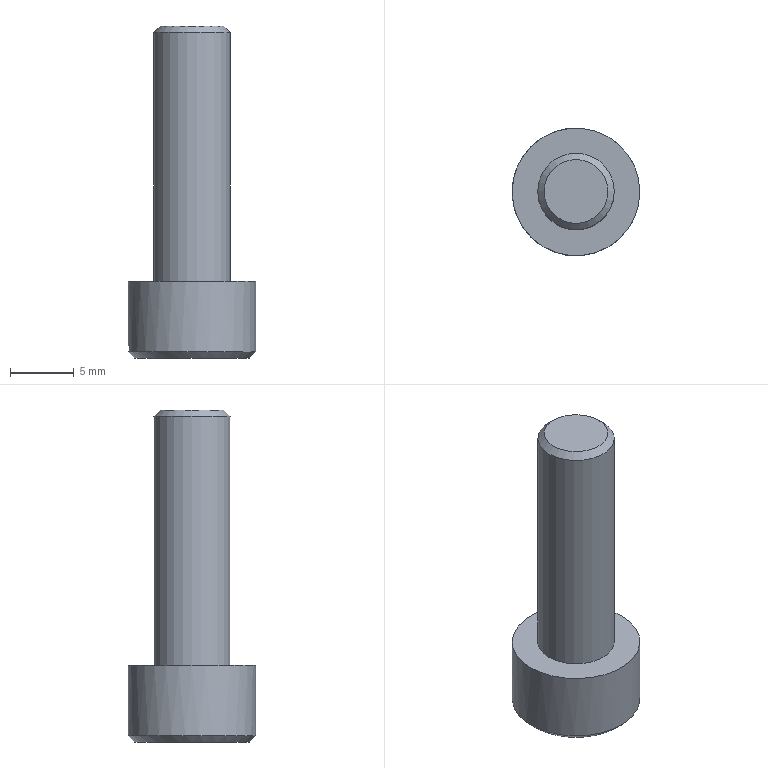Part | STEP file | gslz 2016.10.28-6_id258_x_t | 1 solid | 14 faces | box 10 x 10 x 26 mm | volume 944.102 mm3 | plane 10 | cylinder 2 | cone 2 | commonest cylinder face diameters 6 x1 10 x1
STEP:
#1=CARTESIAN_POINT('',(-78.45,150.,90.992));
#2=VERTEX_POINT('',#1);
#3=CARTESIAN_POINT('',(-82.95,150.,90.992));
#4=DIRECTION('',(0.,0.,1.));
#5=DIRECTION('',(1.,0.,0.));
#6=AXIS2_PLACEMENT_3D('',#3,#4,#5);
#7=CIRCLE('',#6,4.5);
#8=EDGE_CURVE('',#2,#2,#7,.T.);
#9=ORIENTED_EDGE('',*,*,#8,.F.);
#10=EDGE_LOOP('',(#9));
#11=FACE_BOUND('',#10,.T.);
#12=CARTESIAN_POINT('',(-85.45,151.443,90.992));
#13=VERTEX_POINT('',#12);
#14=CARTESIAN_POINT('',(-85.45,148.557,90.992));
#15=VERTEX_POINT('',#14);
#16=CARTESIAN_POINT('',(-85.45,151.443,90.992));
#17=DIRECTION('',(0.,-1.,0.));
#18=VECTOR('',#17,1.);
#19=LINE('',#16,#18);
#20=EDGE_CURVE('',#13,#15,#19,.T.);
#21=ORIENTED_EDGE('',*,*,#20,.T.);
#22=CARTESIAN_POINT('',(-82.95,147.113,90.992));
#23=VERTEX_POINT('',#22);
#24=CARTESIAN_POINT('',(-85.45,148.557,90.992));
#25=DIRECTION('',(0.866,-0.5,0.));
#26=VECTOR('',#25,1.);
#27=LINE('',#24,#26);
#28=EDGE_CURVE('',#15,#23,#27,.T.);
#29=ORIENTED_EDGE('',*,*,#28,.T.);
#30=CARTESIAN_POINT('',(-80.45,148.557,90.992));
#31=VERTEX_POINT('',#30);
#32=CARTESIAN_POINT('',(-82.95,147.113,90.992));
#33=DIRECTION('',(0.866,0.5,0.));
#34=VECTOR('',#33,1.);
#35=LINE('',#32,#34);
#36=EDGE_CURVE('',#23,#31,#35,.T.);
#37=ORIENTED_EDGE('',*,*,#36,.T.);
#38=CARTESIAN_POINT('',(-80.45,151.443,90.992));
#39=VERTEX_POINT('',#38);
#40=CARTESIAN_POINT('',(-80.45,148.557,90.992));
#41=DIRECTION('',(0.,1.,0.));
#42=VECTOR('',#41,1.);
#43=LINE('',#40,#42);
#44=EDGE_CURVE('',#31,#39,#43,.T.);
#45=ORIENTED_EDGE('',*,*,#44,.T.);
#46=CARTESIAN_POINT('',(-82.95,152.887,90.992));
#47=VERTEX_POINT('',#46);
#48=CARTESIAN_POINT('',(-80.45,151.443,90.992));
#49=DIRECTION('',(-0.866,0.5,0.));
#50=VECTOR('',#49,1.);
#51=LINE('',#48,#50);
#52=EDGE_CURVE('',#39,#47,#51,.T.);
#53=ORIENTED_EDGE('',*,*,#52,.T.);
#54=CARTESIAN_POINT('',(-82.95,152.887,90.992));
#55=DIRECTION('',(-0.866,-0.5,0.));
#56=VECTOR('',#55,1.);
#57=LINE('',#54,#56);
#58=EDGE_CURVE('',#47,#13,#57,.T.);
#59=ORIENTED_EDGE('',*,*,#58,.T.);
#60=EDGE_LOOP('',(#21,#29,#37,#45,#53,#59));
#61=FACE_BOUND('',#60,.T.);
#62=CARTESIAN_POINT('',(-82.95,150.,90.992));
#63=DIRECTION('',(0.,0.,-1.));
#64=DIRECTION('',(-1.,0.,0.));
#65=AXIS2_PLACEMENT_3D('',#62,#63,#64);
#66=PLANE('',#65);
#67=ADVANCED_FACE('',(#11,#61),#66,.T.);
#68=CARTESIAN_POINT('',(-85.45,150.,116.992));
#69=VERTEX_POINT('',#68);
#70=CARTESIAN_POINT('',(-82.95,150.,116.992));
#71=DIRECTION('',(0.,0.,-1.));
#72=DIRECTION('',(-1.,0.,0.));
#73=AXIS2_PLACEMENT_3D('',#70,#71,#72);
#74=CIRCLE('',#73,2.5);
#75=EDGE_CURVE('',#69,#69,#74,.T.);
#76=ORIENTED_EDGE('',*,*,#75,.F.);
#77=EDGE_LOOP('',(#76));
#78=FACE_OUTER_BOUND('',#77,.T.);
#79=CARTESIAN_POINT('',(-82.95,150.,116.992));
#80=DIRECTION('',(0.,0.,1.));
#81=DIRECTION('',(1.,0.,0.));
#82=AXIS2_PLACEMENT_3D('',#79,#80,#81);
#83=PLANE('',#82);
#84=ADVANCED_FACE('',(#78),#83,.T.);
#85=CARTESIAN_POINT('',(-79.95,150.,116.492));
#86=VERTEX_POINT('',#85);
#87=CARTESIAN_POINT('',(-82.95,150.,116.492));
#88=DIRECTION('',(0.,0.,1.));
#89=DIRECTION('',(1.,0.,0.));
#90=AXIS2_PLACEMENT_3D('',#87,#88,#89);
#91=CIRCLE('',#90,3.);
#92=EDGE_CURVE('',#86,#86,#91,.T.);
#93=ORIENTED_EDGE('',*,*,#92,.F.);
#94=EDGE_LOOP('',(#93));
#95=FACE_BOUND('',#94,.T.);
#96=CARTESIAN_POINT('',(-85.95,150.,96.992));
#97=VERTEX_POINT('',#96);
#98=CARTESIAN_POINT('',(-82.95,150.,96.992));
#99=DIRECTION('',(0.,0.,-1.));
#100=DIRECTION('',(-1.,0.,0.));
#101=AXIS2_PLACEMENT_3D('',#98,#99,#100);
#102=CIRCLE('',#101,3.);
#103=EDGE_CURVE('',#97,#97,#102,.T.);
#104=ORIENTED_EDGE('',*,*,#103,.F.);
#105=EDGE_LOOP('',(#104));
#106=FACE_BOUND('',#105,.T.);
#107=CARTESIAN_POINT('',(-82.95,150.,108.992));
#108=DIRECTION('',(0.,0.,1.));
#109=DIRECTION('',(1.,0.,0.));
#110=AXIS2_PLACEMENT_3D('',#107,#108,#109);
#111=CYLINDRICAL_SURFACE('',#110,3.);
#112=ADVANCED_FACE('',(#95,#106),#111,.T.);
#113=ORIENTED_EDGE('',*,*,#103,.T.);
#114=EDGE_LOOP('',(#113));
#115=FACE_BOUND('',#114,.T.);
#116=CARTESIAN_POINT('',(-87.95,150.,96.992));
#117=VERTEX_POINT('',#116);
#118=CARTESIAN_POINT('',(-82.95,150.,96.992));
#119=DIRECTION('',(0.,0.,-1.));
#120=DIRECTION('',(-1.,0.,0.));
#121=AXIS2_PLACEMENT_3D('',#118,#119,#120);
#122=CIRCLE('',#121,5.);
#123=EDGE_CURVE('',#117,#117,#122,.T.);
#124=ORIENTED_EDGE('',*,*,#123,.F.);
#125=EDGE_LOOP('',(#124));
#126=FACE_BOUND('',#125,.T.);
#127=CARTESIAN_POINT('',(-82.95,150.,96.992));
#128=DIRECTION('',(0.,0.,1.));
#129=DIRECTION('',(1.,0.,0.));
#130=AXIS2_PLACEMENT_3D('',#127,#128,#129);
#131=PLANE('',#130);
#132=ADVANCED_FACE('',(#115,#126),#131,.T.);
#133=CARTESIAN_POINT('',(-77.95,150.,91.492));
#134=VERTEX_POINT('',#133);
#135=CARTESIAN_POINT('',(-82.95,150.,91.492));
#136=DIRECTION('',(0.,0.,-1.));
#137=DIRECTION('',(1.,0.,0.));
#138=AXIS2_PLACEMENT_3D('',#135,#136,#137);
#139=CIRCLE('',#138,5.);
#140=EDGE_CURVE('',#134,#134,#139,.T.);
#141=ORIENTED_EDGE('',*,*,#140,.F.);
#142=EDGE_LOOP('',(#141));
#143=FACE_BOUND('',#142,.T.);
#144=ORIENTED_EDGE('',*,*,#123,.T.);
#145=EDGE_LOOP('',(#144));
#146=FACE_BOUND('',#145,.T.);
#147=CARTESIAN_POINT('',(-82.95,150.,88.992));
#148=DIRECTION('',(0.,0.,1.));
#149=DIRECTION('',(1.,0.,0.));
#150=AXIS2_PLACEMENT_3D('',#147,#148,#149);
#151=CYLINDRICAL_SURFACE('',#150,5.);
#152=ADVANCED_FACE('',(#143,#146),#151,.T.);
#153=ORIENTED_EDGE('',*,*,#92,.T.);
#154=EDGE_LOOP('',(#153));
#155=FACE_BOUND('',#154,.T.);
#156=ORIENTED_EDGE('',*,*,#75,.T.);
#157=EDGE_LOOP('',(#156));
#158=FACE_BOUND('',#157,.T.);
#159=CARTESIAN_POINT('',(-82.95,150.,116.992));
#160=DIRECTION('',(0.,0.,-1.));
#161=DIRECTION('',(1.,0.,0.));
#162=AXIS2_PLACEMENT_3D('',#159,#160,#161);
#163=CONICAL_SURFACE('',#162,2.5,45.);
#164=ADVANCED_FACE('',(#155,#158),#163,.T.);
#165=ORIENTED_EDGE('',*,*,#20,.F.);
#166=CARTESIAN_POINT('',(-85.45,151.443,94.992));
#167=VERTEX_POINT('',#166);
#168=CARTESIAN_POINT('',(-85.45,151.443,94.992));
#169=DIRECTION('',(0.,0.,1.));
#170=VECTOR('',#169,1.);
#171=LINE('',#168,#170);
#172=EDGE_CURVE('',#13,#167,#171,.T.);
#173=ORIENTED_EDGE('',*,*,#172,.T.);
#174=CARTESIAN_POINT('',(-85.45,148.557,94.992));
#175=VERTEX_POINT('',#174);
#176=CARTESIAN_POINT('',(-85.45,151.443,94.992));
#177=DIRECTION('',(0.,1.,0.));
#178=VECTOR('',#177,1.);
#179=LINE('',#176,#178);
#180=EDGE_CURVE('',#175,#167,#179,.T.);
#181=ORIENTED_EDGE('',*,*,#180,.F.);
#182=CARTESIAN_POINT('',(-85.45,148.557,94.992));
#183=DIRECTION('',(0.,0.,1.));
#184=VECTOR('',#183,1.);
#185=LINE('',#182,#184);
#186=EDGE_CURVE('',#15,#175,#185,.T.);
#187=ORIENTED_EDGE('',*,*,#186,.F.);
#188=EDGE_LOOP('',(#165,#173,#181,#187));
#189=FACE_OUTER_BOUND('',#188,.T.);
#190=CARTESIAN_POINT('',(-85.45,151.443,94.992));
#191=DIRECTION('',(-1.,0.,0.));
#192=DIRECTION('',(0.,0.,1.));
#193=AXIS2_PLACEMENT_3D('',#190,#191,#192);
#194=PLANE('',#193);
#195=ADVANCED_FACE('',(#189),#194,.F.);
#196=ORIENTED_EDGE('',*,*,#28,.F.);
#197=ORIENTED_EDGE('',*,*,#186,.T.);
#198=CARTESIAN_POINT('',(-82.95,147.113,94.992));
#199=VERTEX_POINT('',#198);
#200=CARTESIAN_POINT('',(-85.45,148.557,94.992));
#201=DIRECTION('',(-0.866,0.5,0.));
#202=VECTOR('',#201,1.);
#203=LINE('',#200,#202);
#204=EDGE_CURVE('',#199,#175,#203,.T.);
#205=ORIENTED_EDGE('',*,*,#204,.F.);
#206=CARTESIAN_POINT('',(-82.95,147.113,94.992));
#207=DIRECTION('',(0.,0.,1.));
#208=VECTOR('',#207,1.);
#209=LINE('',#206,#208);
#210=EDGE_CURVE('',#23,#199,#209,.T.);
#211=ORIENTED_EDGE('',*,*,#210,.F.);
#212=EDGE_LOOP('',(#196,#197,#205,#211));
#213=FACE_OUTER_BOUND('',#212,.T.);
#214=CARTESIAN_POINT('',(-85.45,148.557,94.992));
#215=DIRECTION('',(-0.5,-0.866,0.));
#216=DIRECTION('',(-0.866,0.5,0.));
#217=AXIS2_PLACEMENT_3D('',#214,#215,#216);
#218=PLANE('',#217);
#219=ADVANCED_FACE('',(#213),#218,.F.);
#220=ORIENTED_EDGE('',*,*,#36,.F.);
#221=ORIENTED_EDGE('',*,*,#210,.T.);
#222=CARTESIAN_POINT('',(-80.45,148.557,94.992));
#223=VERTEX_POINT('',#222);
#224=CARTESIAN_POINT('',(-82.95,147.113,94.992));
#225=DIRECTION('',(-0.866,-0.5,0.));
#226=VECTOR('',#225,1.);
#227=LINE('',#224,#226);
#228=EDGE_CURVE('',#223,#199,#227,.T.);
#229=ORIENTED_EDGE('',*,*,#228,.F.);
#230=CARTESIAN_POINT('',(-80.45,148.557,94.992));
#231=DIRECTION('',(0.,0.,1.));
#232=VECTOR('',#231,1.);
#233=LINE('',#230,#232);
#234=EDGE_CURVE('',#31,#223,#233,.T.);
#235=ORIENTED_EDGE('',*,*,#234,.F.);
#236=EDGE_LOOP('',(#220,#221,#229,#235));
#237=FACE_OUTER_BOUND('',#236,.T.);
#238=CARTESIAN_POINT('',(-82.95,147.113,94.992));
#239=DIRECTION('',(0.5,-0.866,0.));
#240=DIRECTION('',(-0.866,-0.5,0.));
#241=AXIS2_PLACEMENT_3D('',#238,#239,#240);
#242=PLANE('',#241);
#243=ADVANCED_FACE('',(#237),#242,.F.);
#244=ORIENTED_EDGE('',*,*,#44,.F.);
#245=ORIENTED_EDGE('',*,*,#234,.T.);
#246=CARTESIAN_POINT('',(-80.45,151.443,94.992));
#247=VERTEX_POINT('',#246);
#248=CARTESIAN_POINT('',(-80.45,148.557,94.992));
#249=DIRECTION('',(0.,-1.,0.));
#250=VECTOR('',#249,1.);
#251=LINE('',#248,#250);
#252=EDGE_CURVE('',#247,#223,#251,.T.);
#253=ORIENTED_EDGE('',*,*,#252,.F.);
#254=CARTESIAN_POINT('',(-80.45,151.443,94.992));
#255=DIRECTION('',(0.,0.,1.));
#256=VECTOR('',#255,1.);
#257=LINE('',#254,#256);
#258=EDGE_CURVE('',#39,#247,#257,.T.);
#259=ORIENTED_EDGE('',*,*,#258,.F.);
#260=EDGE_LOOP('',(#244,#245,#253,#259));
#261=FACE_OUTER_BOUND('',#260,.T.);
#262=CARTESIAN_POINT('',(-80.45,148.557,94.992));
#263=DIRECTION('',(1.,0.,0.));
#264=DIRECTION('',(0.,0.,-1.));
#265=AXIS2_PLACEMENT_3D('',#262,#263,#264);
#266=PLANE('',#265);
#267=ADVANCED_FACE('',(#261),#266,.F.);
#268=ORIENTED_EDGE('',*,*,#52,.F.);
#269=ORIENTED_EDGE('',*,*,#258,.T.);
#270=CARTESIAN_POINT('',(-82.95,152.887,94.992));
#271=VERTEX_POINT('',#270);
#272=CARTESIAN_POINT('',(-80.45,151.443,94.992));
#273=DIRECTION('',(0.866,-0.5,0.));
#274=VECTOR('',#273,1.);
#275=LINE('',#272,#274);
#276=EDGE_CURVE('',#271,#247,#275,.T.);
#277=ORIENTED_EDGE('',*,*,#276,.F.);
#278=CARTESIAN_POINT('',(-82.95,152.887,94.992));
#279=DIRECTION('',(0.,0.,1.));
#280=VECTOR('',#279,1.);
#281=LINE('',#278,#280);
#282=EDGE_CURVE('',#47,#271,#281,.T.);
#283=ORIENTED_EDGE('',*,*,#282,.F.);
#284=EDGE_LOOP('',(#268,#269,#277,#283));
#285=FACE_OUTER_BOUND('',#284,.T.);
#286=CARTESIAN_POINT('',(-80.45,151.443,94.992));
#287=DIRECTION('',(0.5,0.866,0.));
#288=DIRECTION('',(0.866,-0.5,0.));
#289=AXIS2_PLACEMENT_3D('',#286,#287,#288);
#290=PLANE('',#289);
#291=ADVANCED_FACE('',(#285),#290,.F.);
#292=ORIENTED_EDGE('',*,*,#58,.F.);
#293=ORIENTED_EDGE('',*,*,#282,.T.);
#294=CARTESIAN_POINT('',(-82.95,152.887,94.992));
#295=DIRECTION('',(0.866,0.5,0.));
#296=VECTOR('',#295,1.);
#297=LINE('',#294,#296);
#298=EDGE_CURVE('',#167,#271,#297,.T.);
#299=ORIENTED_EDGE('',*,*,#298,.F.);
#300=ORIENTED_EDGE('',*,*,#172,.F.);
#301=EDGE_LOOP('',(#292,#293,#299,#300));
#302=FACE_OUTER_BOUND('',#301,.T.);
#303=CARTESIAN_POINT('',(-82.95,152.887,94.992));
#304=DIRECTION('',(-0.5,0.866,0.));
#305=DIRECTION('',(0.866,0.5,0.));
#306=AXIS2_PLACEMENT_3D('',#303,#304,#305);
#307=PLANE('',#306);
#308=ADVANCED_FACE('',(#302),#307,.F.);
#309=ORIENTED_EDGE('',*,*,#180,.T.);
#310=ORIENTED_EDGE('',*,*,#298,.T.);
#311=ORIENTED_EDGE('',*,*,#276,.T.);
#312=ORIENTED_EDGE('',*,*,#252,.T.);
#313=ORIENTED_EDGE('',*,*,#228,.T.);
#314=ORIENTED_EDGE('',*,*,#204,.T.);
#315=EDGE_LOOP('',(#309,#310,#311,#312,#313,#314));
#316=FACE_OUTER_BOUND('',#315,.T.);
#317=CARTESIAN_POINT('',(-85.45,148.557,94.992));
#318=DIRECTION('',(0.,0.,-1.));
#319=DIRECTION('',(-1.,0.,0.));
#320=AXIS2_PLACEMENT_3D('',#317,#318,#319);
#321=PLANE('',#320);
#322=ADVANCED_FACE('',(#316),#321,.T.);
#323=ORIENTED_EDGE('',*,*,#8,.T.);
#324=EDGE_LOOP('',(#323));
#325=FACE_BOUND('',#324,.T.);
#326=ORIENTED_EDGE('',*,*,#140,.T.);
#327=EDGE_LOOP('',(#326));
#328=FACE_BOUND('',#327,.T.);
#329=CARTESIAN_POINT('',(-82.95,150.,91.492));
#330=DIRECTION('',(0.,0.,1.));
#331=DIRECTION('',(1.,0.,0.));
#332=AXIS2_PLACEMENT_3D('',#329,#330,#331);
#333=CONICAL_SURFACE('',#332,5.,45.);
#334=ADVANCED_FACE('',(#325,#328),#333,.T.);
#335=CLOSED_SHELL('',(#67,#84,#112,#132,#152,#164,#195,#219,#243,#267,#291,#308,#322,#334));
#336=MANIFOLD_SOLID_BREP('',#335);
#337=(LENGTH_UNIT()NAMED_UNIT(*)SI_UNIT(.MILLI.,.METRE.));
#338=UNCERTAINTY_MEASURE_WITH_UNIT(LENGTH_MEASURE(0.00002),#337,'','');
#339=(NAMED_UNIT(*)PLANE_ANGLE_UNIT()SI_UNIT($,.RADIAN.));
#340=PLANE_ANGLE_MEASURE_WITH_UNIT(PLANE_ANGLE_MEASURE(0.01745),#339);
#341=DIMENSIONAL_EXPONENTS(0.,0.,0.,0.,0.,0.,0.);
#342=(CONVERSION_BASED_UNIT('DEGREE',#340)NAMED_UNIT(#341)PLANE_ANGLE_UNIT());
#343=(NAMED_UNIT(*)SI_UNIT($,.STERADIAN.)SOLID_ANGLE_UNIT());
#344=(GEOMETRIC_REPRESENTATION_CONTEXT(3)GLOBAL_UNCERTAINTY_ASSIGNED_CONTEXT((#338))GLOBAL_UNIT_ASSIGNED_CONTEXT((#337,#342,#343))REPRESENTATION_CONTEXT('',''));
#345=ADVANCED_BREP_SHAPE_REPRESENTATION('',(#336),#344);